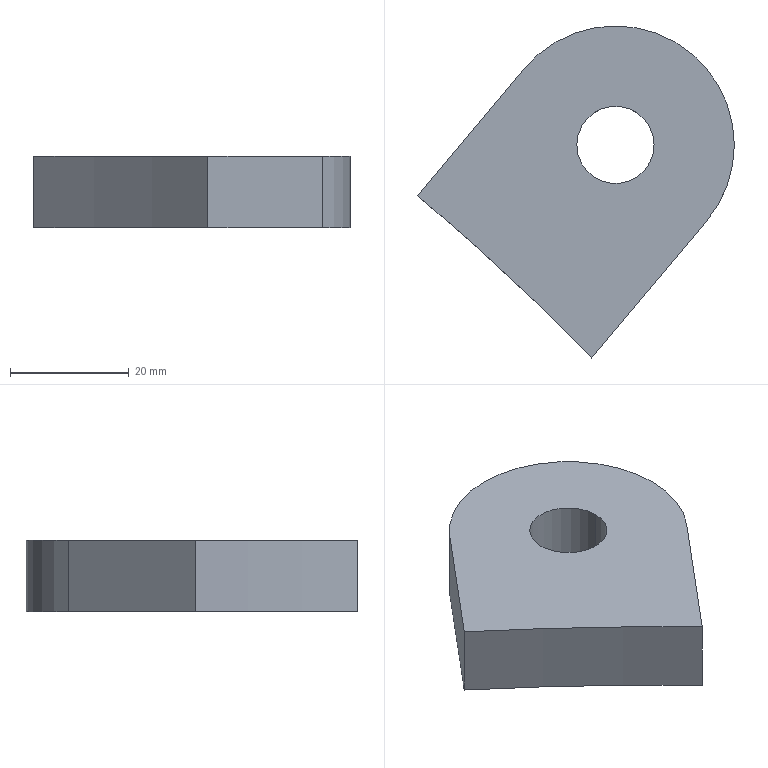Part | SolidWorks | features Extrusion 1 | 1 solid | 8 faces | box 53.274 x 55.837 x 12 mm | volume 19684 mm3 | cylinder 4 | plane 4 | commonest cylinder face diameters 13 x2 40 x1 775 x1
STEP:
#1=CARTESIAN_POINT('',(275.854,305.382,6.));
#2=VERTEX_POINT('',#1);
#3=CARTESIAN_POINT('',(288.854,305.382,6.));
#4=VERTEX_POINT('',#3);
#5=CARTESIAN_POINT('',(282.354,305.382,6.));
#6=DIRECTION('',(0.,0.,1.));
#7=DIRECTION('',(1.,0.,0.));
#8=AXIS2_PLACEMENT_3D('',#5,#6,#7);
#9=CIRCLE('',#8,6.5);
#10=EDGE_CURVE('',#2,#4,#9,.T.);
#11=ORIENTED_EDGE('',*,*,#10,.T.);
#12=CARTESIAN_POINT('',(288.854,305.382,-6.));
#13=VERTEX_POINT('',#12);
#14=CARTESIAN_POINT('',(288.854,305.382,6.));
#15=DIRECTION('',(0.,0.,-1.));
#16=VECTOR('',#15,1000.);
#17=LINE('',#14,#16);
#18=EDGE_CURVE('',#4,#13,#17,.T.);
#19=ORIENTED_EDGE('',*,*,#18,.T.);
#20=CARTESIAN_POINT('',(275.854,305.382,-6.));
#21=VERTEX_POINT('',#20);
#22=CARTESIAN_POINT('',(282.354,305.382,-6.));
#23=DIRECTION('',(0.,0.,1.));
#24=DIRECTION('',(1.,0.,0.));
#25=AXIS2_PLACEMENT_3D('',#22,#23,#24);
#26=CIRCLE('',#25,6.5);
#27=EDGE_CURVE('',#21,#13,#26,.T.);
#28=ORIENTED_EDGE('',*,*,#27,.F.);
#29=CARTESIAN_POINT('',(275.854,305.382,6.));
#30=DIRECTION('',(0.,0.,-1.));
#31=VECTOR('',#30,1000.);
#32=LINE('',#29,#31);
#33=EDGE_CURVE('',#2,#21,#32,.T.);
#34=ORIENTED_EDGE('',*,*,#33,.F.);
#35=EDGE_LOOP('',(#11,#19,#28,#34));
#36=FACE_OUTER_BOUND('',#35,.T.);
#37=CARTESIAN_POINT('',(282.354,305.382,6.));
#38=DIRECTION('',(0.,0.,-1.));
#39=DIRECTION('',(-1.,0.,0.));
#40=AXIS2_PLACEMENT_3D('',#37,#38,#39);
#41=CYLINDRICAL_SURFACE('',#40,6.5);
#42=ADVANCED_FACE('',(#36),#41,.F.);
#43=CARTESIAN_POINT('',(249.08,296.842,6.));
#44=VERTEX_POINT('',#43);
#45=CARTESIAN_POINT('',(278.391,269.545,6.));
#46=VERTEX_POINT('',#45);
#47=CARTESIAN_POINT('',(0.,0.,6.));
#48=DIRECTION('',(0.,0.,-1.));
#49=DIRECTION('',(-1.,0.,0.));
#50=AXIS2_PLACEMENT_3D('',#47,#48,#49);
#51=CIRCLE('',#50,387.5);
#52=EDGE_CURVE('',#44,#46,#51,.T.);
#53=ORIENTED_EDGE('',*,*,#52,.T.);
#54=CARTESIAN_POINT('',(297.675,292.526,6.));
#55=VERTEX_POINT('',#54);
#56=CARTESIAN_POINT('',(278.391,269.545,6.));
#57=DIRECTION('',(0.6428,0.766,0.));
#58=VECTOR('',#57,1000.);
#59=LINE('',#56,#58);
#60=EDGE_CURVE('',#46,#55,#59,.T.);
#61=ORIENTED_EDGE('',*,*,#60,.T.);
#62=CARTESIAN_POINT('',(267.033,318.238,6.));
#63=VERTEX_POINT('',#62);
#64=CARTESIAN_POINT('',(282.354,305.382,6.));
#65=DIRECTION('',(0.,0.,1.));
#66=DIRECTION('',(-1.,0.,0.));
#67=AXIS2_PLACEMENT_3D('',#64,#65,#66);
#68=CIRCLE('',#67,20.);
#69=EDGE_CURVE('',#55,#63,#68,.T.);
#70=ORIENTED_EDGE('',*,*,#69,.T.);
#71=CARTESIAN_POINT('',(249.08,296.842,6.));
#72=DIRECTION('',(-0.6428,-0.766,0.));
#73=VECTOR('',#72,1000.);
#74=LINE('',#71,#73);
#75=EDGE_CURVE('',#63,#44,#74,.T.);
#76=ORIENTED_EDGE('',*,*,#75,.T.);
#77=EDGE_LOOP('',(#53,#61,#70,#76));
#78=FACE_OUTER_BOUND('',#77,.T.);
#79=ORIENTED_EDGE('',*,*,#10,.F.);
#80=CARTESIAN_POINT('',(282.354,305.382,6.));
#81=DIRECTION('',(0.,0.,1.));
#82=DIRECTION('',(1.,0.,0.));
#83=AXIS2_PLACEMENT_3D('',#80,#81,#82);
#84=CIRCLE('',#83,6.5);
#85=EDGE_CURVE('',#4,#2,#84,.T.);
#86=ORIENTED_EDGE('',*,*,#85,.F.);
#87=EDGE_LOOP('',(#79,#86));
#88=FACE_BOUND('',#87,.T.);
#89=CARTESIAN_POINT('',(0.,0.,6.));
#90=DIRECTION('',(0.,0.,-1.));
#91=DIRECTION('',(-1.,0.,0.));
#92=AXIS2_PLACEMENT_3D('',#89,#90,#91);
#93=PLANE('',#92);
#94=ADVANCED_FACE('',(#78,#88),#93,.F.);
#95=CARTESIAN_POINT('',(249.08,296.842,-6.));
#96=VERTEX_POINT('',#95);
#97=CARTESIAN_POINT('',(278.391,269.545,-6.));
#98=VERTEX_POINT('',#97);
#99=CARTESIAN_POINT('',(0.,0.,-6.));
#100=DIRECTION('',(0.,0.,-1.));
#101=DIRECTION('',(-1.,0.,0.));
#102=AXIS2_PLACEMENT_3D('',#99,#100,#101);
#103=CIRCLE('',#102,387.5);
#104=EDGE_CURVE('',#96,#98,#103,.T.);
#105=ORIENTED_EDGE('',*,*,#104,.F.);
#106=CARTESIAN_POINT('',(267.033,318.238,-6.));
#107=VERTEX_POINT('',#106);
#108=CARTESIAN_POINT('',(249.08,296.842,-6.));
#109=DIRECTION('',(-0.6428,-0.766,0.));
#110=VECTOR('',#109,1000.);
#111=LINE('',#108,#110);
#112=EDGE_CURVE('',#107,#96,#111,.T.);
#113=ORIENTED_EDGE('',*,*,#112,.F.);
#114=CARTESIAN_POINT('',(297.675,292.526,-6.));
#115=VERTEX_POINT('',#114);
#116=CARTESIAN_POINT('',(282.354,305.382,-6.));
#117=DIRECTION('',(0.,0.,1.));
#118=DIRECTION('',(-1.,0.,0.));
#119=AXIS2_PLACEMENT_3D('',#116,#117,#118);
#120=CIRCLE('',#119,20.);
#121=EDGE_CURVE('',#115,#107,#120,.T.);
#122=ORIENTED_EDGE('',*,*,#121,.F.);
#123=CARTESIAN_POINT('',(278.391,269.545,-6.));
#124=DIRECTION('',(0.6428,0.766,0.));
#125=VECTOR('',#124,1000.);
#126=LINE('',#123,#125);
#127=EDGE_CURVE('',#98,#115,#126,.T.);
#128=ORIENTED_EDGE('',*,*,#127,.F.);
#129=EDGE_LOOP('',(#105,#113,#122,#128));
#130=FACE_OUTER_BOUND('',#129,.T.);
#131=ORIENTED_EDGE('',*,*,#27,.T.);
#132=CARTESIAN_POINT('',(282.354,305.382,-6.));
#133=DIRECTION('',(0.,0.,1.));
#134=DIRECTION('',(1.,0.,0.));
#135=AXIS2_PLACEMENT_3D('',#132,#133,#134);
#136=CIRCLE('',#135,6.5);
#137=EDGE_CURVE('',#13,#21,#136,.T.);
#138=ORIENTED_EDGE('',*,*,#137,.T.);
#139=EDGE_LOOP('',(#131,#138));
#140=FACE_BOUND('',#139,.T.);
#141=CARTESIAN_POINT('',(0.,0.,-6.));
#142=DIRECTION('',(0.,0.,-1.));
#143=DIRECTION('',(-1.,0.,0.));
#144=AXIS2_PLACEMENT_3D('',#141,#142,#143);
#145=PLANE('',#144);
#146=ADVANCED_FACE('',(#130,#140),#145,.T.);
#147=ORIENTED_EDGE('',*,*,#104,.T.);
#148=CARTESIAN_POINT('',(278.391,269.545,6.));
#149=DIRECTION('',(0.,0.,-1.));
#150=VECTOR('',#149,1000.);
#151=LINE('',#148,#150);
#152=EDGE_CURVE('',#46,#98,#151,.T.);
#153=ORIENTED_EDGE('',*,*,#152,.F.);
#154=ORIENTED_EDGE('',*,*,#52,.F.);
#155=CARTESIAN_POINT('',(249.08,296.842,6.));
#156=DIRECTION('',(0.,0.,-1.));
#157=VECTOR('',#156,1000.);
#158=LINE('',#155,#157);
#159=EDGE_CURVE('',#44,#96,#158,.T.);
#160=ORIENTED_EDGE('',*,*,#159,.T.);
#161=EDGE_LOOP('',(#147,#153,#154,#160));
#162=FACE_OUTER_BOUND('',#161,.T.);
#163=CARTESIAN_POINT('',(0.,0.,6.));
#164=DIRECTION('',(0.,0.,-1.));
#165=DIRECTION('',(-1.,0.,0.));
#166=AXIS2_PLACEMENT_3D('',#163,#164,#165);
#167=CYLINDRICAL_SURFACE('',#166,387.5);
#168=ADVANCED_FACE('',(#162),#167,.F.);
#169=ORIENTED_EDGE('',*,*,#127,.T.);
#170=CARTESIAN_POINT('',(297.675,292.526,6.));
#171=DIRECTION('',(0.,0.,-1.));
#172=VECTOR('',#171,1000.);
#173=LINE('',#170,#172);
#174=EDGE_CURVE('',#55,#115,#173,.T.);
#175=ORIENTED_EDGE('',*,*,#174,.F.);
#176=ORIENTED_EDGE('',*,*,#60,.F.);
#177=ORIENTED_EDGE('',*,*,#152,.T.);
#178=EDGE_LOOP('',(#169,#175,#176,#177));
#179=FACE_OUTER_BOUND('',#178,.T.);
#180=CARTESIAN_POINT('',(278.391,269.545,6.));
#181=DIRECTION('',(-0.766,0.6428,0.));
#182=DIRECTION('',(-0.6428,-0.766,0.));
#183=AXIS2_PLACEMENT_3D('',#180,#181,#182);
#184=PLANE('',#183);
#185=ADVANCED_FACE('',(#179),#184,.F.);
#186=ORIENTED_EDGE('',*,*,#121,.T.);
#187=CARTESIAN_POINT('',(267.033,318.238,6.));
#188=DIRECTION('',(0.,0.,-1.));
#189=VECTOR('',#188,1000.);
#190=LINE('',#187,#189);
#191=EDGE_CURVE('',#63,#107,#190,.T.);
#192=ORIENTED_EDGE('',*,*,#191,.F.);
#193=ORIENTED_EDGE('',*,*,#69,.F.);
#194=ORIENTED_EDGE('',*,*,#174,.T.);
#195=EDGE_LOOP('',(#186,#192,#193,#194));
#196=FACE_OUTER_BOUND('',#195,.T.);
#197=CARTESIAN_POINT('',(282.354,305.382,6.));
#198=DIRECTION('',(0.,0.,-1.));
#199=DIRECTION('',(-1.,0.,0.));
#200=AXIS2_PLACEMENT_3D('',#197,#198,#199);
#201=CYLINDRICAL_SURFACE('',#200,20.);
#202=ADVANCED_FACE('',(#196),#201,.T.);
#203=ORIENTED_EDGE('',*,*,#112,.T.);
#204=ORIENTED_EDGE('',*,*,#159,.F.);
#205=ORIENTED_EDGE('',*,*,#75,.F.);
#206=ORIENTED_EDGE('',*,*,#191,.T.);
#207=EDGE_LOOP('',(#203,#204,#205,#206));
#208=FACE_OUTER_BOUND('',#207,.T.);
#209=CARTESIAN_POINT('',(249.08,296.842,6.));
#210=DIRECTION('',(0.766,-0.6428,0.));
#211=DIRECTION('',(0.6428,0.766,0.));
#212=AXIS2_PLACEMENT_3D('',#209,#210,#211);
#213=PLANE('',#212);
#214=ADVANCED_FACE('',(#208),#213,.F.);
#215=ORIENTED_EDGE('',*,*,#18,.F.);
#216=ORIENTED_EDGE('',*,*,#85,.T.);
#217=ORIENTED_EDGE('',*,*,#33,.T.);
#218=ORIENTED_EDGE('',*,*,#137,.F.);
#219=EDGE_LOOP('',(#215,#216,#217,#218));
#220=FACE_OUTER_BOUND('',#219,.T.);
#221=CARTESIAN_POINT('',(282.354,305.382,6.));
#222=DIRECTION('',(0.,0.,-1.));
#223=DIRECTION('',(-1.,0.,0.));
#224=AXIS2_PLACEMENT_3D('',#221,#222,#223);
#225=CYLINDRICAL_SURFACE('',#224,6.5);
#226=ADVANCED_FACE('',(#220),#225,.F.);
#227=CLOSED_SHELL('',(#42,#94,#146,#168,#185,#202,#214,#226));
#228=MANIFOLD_SOLID_BREP('',#227);
#229=CARTESIAN_POINT('',(0.,0.,0.));
#230=DIRECTION('',(0.,0.,1.));
#231=DIRECTION('',(1.,0.,0.));
#232=AXIS2_PLACEMENT_3D('',#229,#230,#231);
#233=(LENGTH_UNIT()NAMED_UNIT(*)SI_UNIT(.MILLI.,.METRE.));
#234=UNCERTAINTY_MEASURE_WITH_UNIT(LENGTH_MEASURE(0.00001),#233,'','');
#235=(NAMED_UNIT(*)PLANE_ANGLE_UNIT()SI_UNIT($,.RADIAN.));
#236=(NAMED_UNIT(*)SI_UNIT($,.STERADIAN.)SOLID_ANGLE_UNIT());
#237=(GEOMETRIC_REPRESENTATION_CONTEXT(3)GLOBAL_UNCERTAINTY_ASSIGNED_CONTEXT((#234))GLOBAL_UNIT_ASSIGNED_CONTEXT((#233,#235,#236))REPRESENTATION_CONTEXT('',''));
#238=ADVANCED_BREP_SHAPE_REPRESENTATION('',(#228,#232),#237);